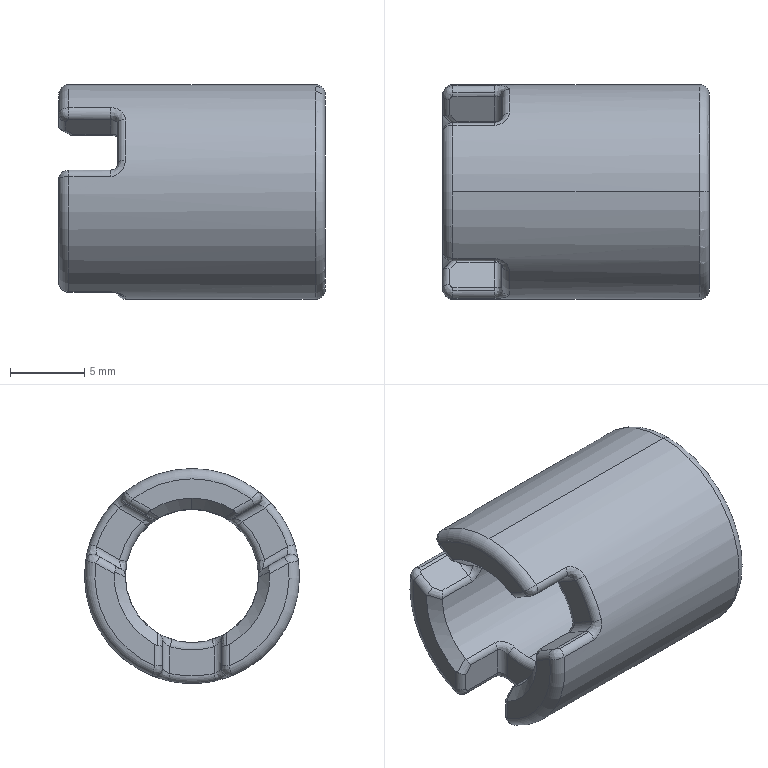Part | NX | features BREP 1 | 1 solid | 86 faces | box 18 x 14.5 x 14.5 mm | volume 1667 mm3 | cylinder 32 | spline 24 | plane 13 | torus 11 | cone 6 | commonest cylinder face diameters 1 x28 9 x2 14.5 x2